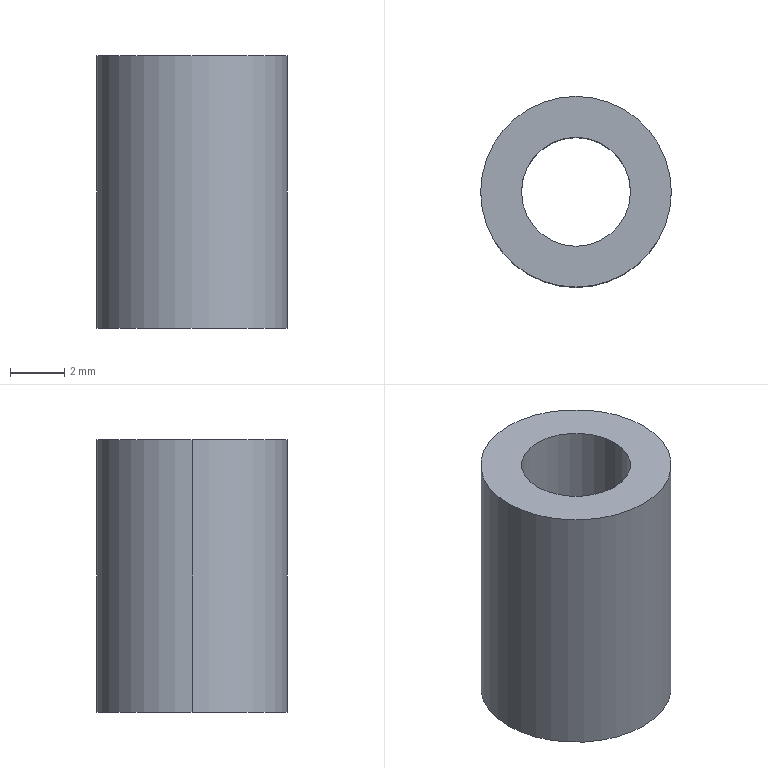Part | STEP file | MANIFOLD_SOLID_BREP_312481-2 | 1 solid | 6 faces | box 7 x 7 x 10 mm | volume 259.181 mm3 | cylinder 4 | plane 2 | commonest cylinder face diameters 4 x2 7 x2
STEP:
#1=CARTESIAN_POINT('',(-23.5,58.,-348.));
#2=VERTEX_POINT('',#1);
#3=CARTESIAN_POINT('',(-16.5,58.,-348.));
#4=VERTEX_POINT('',#3);
#5=CARTESIAN_POINT('',(-20.,58.,-348.));
#6=DIRECTION('',(0.,0.,-1.));
#7=DIRECTION('',(-1.,0.,0.));
#8=AXIS2_PLACEMENT_3D('',#5,#6,#7);
#9=CIRCLE('',#8,3.5);
#10=EDGE_CURVE('',#2,#4,#9,.T.);
#11=ORIENTED_EDGE('',*,*,#10,.T.);
#12=CARTESIAN_POINT('',(-16.5,58.,-358.));
#13=VERTEX_POINT('',#12);
#14=CARTESIAN_POINT('',(-16.5,58.,-348.));
#15=DIRECTION('',(0.,0.,-1.));
#16=VECTOR('',#15,1000.);
#17=LINE('',#14,#16);
#18=EDGE_CURVE('',#4,#13,#17,.T.);
#19=ORIENTED_EDGE('',*,*,#18,.T.);
#20=CARTESIAN_POINT('',(-23.5,58.,-358.));
#21=VERTEX_POINT('',#20);
#22=CARTESIAN_POINT('',(-20.,58.,-358.));
#23=DIRECTION('',(0.,0.,1.));
#24=DIRECTION('',(-1.,0.,0.));
#25=AXIS2_PLACEMENT_3D('',#22,#23,#24);
#26=CIRCLE('',#25,3.5);
#27=EDGE_CURVE('',#13,#21,#26,.T.);
#28=ORIENTED_EDGE('',*,*,#27,.T.);
#29=CARTESIAN_POINT('',(-23.5,58.,-348.));
#30=DIRECTION('',(0.,0.,-1.));
#31=VECTOR('',#30,1000.);
#32=LINE('',#29,#31);
#33=EDGE_CURVE('',#2,#21,#32,.T.);
#34=ORIENTED_EDGE('',*,*,#33,.F.);
#35=EDGE_LOOP('',(#11,#19,#28,#34));
#36=FACE_OUTER_BOUND('',#35,.T.);
#37=CARTESIAN_POINT('',(-20.,58.,-348.));
#38=DIRECTION('',(0.,0.,-1.));
#39=DIRECTION('',(-1.,0.,0.));
#40=AXIS2_PLACEMENT_3D('',#37,#38,#39);
#41=CYLINDRICAL_SURFACE('',#40,3.5);
#42=ADVANCED_FACE('',(#36),#41,.T.);
#43=CARTESIAN_POINT('',(-18.,58.,-348.));
#44=VERTEX_POINT('',#43);
#45=CARTESIAN_POINT('',(-22.,58.,-348.));
#46=VERTEX_POINT('',#45);
#47=CARTESIAN_POINT('',(-20.,58.,-348.));
#48=DIRECTION('',(0.,0.,-1.));
#49=DIRECTION('',(-1.,0.,0.));
#50=AXIS2_PLACEMENT_3D('',#47,#48,#49);
#51=CIRCLE('',#50,2.);
#52=EDGE_CURVE('',#44,#46,#51,.T.);
#53=ORIENTED_EDGE('',*,*,#52,.F.);
#54=CARTESIAN_POINT('',(-18.,58.,-358.));
#55=VERTEX_POINT('',#54);
#56=CARTESIAN_POINT('',(-18.,58.,-348.));
#57=DIRECTION('',(0.,0.,-1.));
#58=VECTOR('',#57,1000.);
#59=LINE('',#56,#58);
#60=EDGE_CURVE('',#44,#55,#59,.T.);
#61=ORIENTED_EDGE('',*,*,#60,.T.);
#62=CARTESIAN_POINT('',(-22.,58.,-358.));
#63=VERTEX_POINT('',#62);
#64=CARTESIAN_POINT('',(-20.,58.,-358.));
#65=DIRECTION('',(0.,0.,-1.));
#66=DIRECTION('',(-1.,0.,0.));
#67=AXIS2_PLACEMENT_3D('',#64,#65,#66);
#68=CIRCLE('',#67,2.);
#69=EDGE_CURVE('',#55,#63,#68,.T.);
#70=ORIENTED_EDGE('',*,*,#69,.T.);
#71=CARTESIAN_POINT('',(-22.,58.,-348.));
#72=DIRECTION('',(0.,0.,-1.));
#73=VECTOR('',#72,1000.);
#74=LINE('',#71,#73);
#75=EDGE_CURVE('',#46,#63,#74,.T.);
#76=ORIENTED_EDGE('',*,*,#75,.F.);
#77=EDGE_LOOP('',(#53,#61,#70,#76));
#78=FACE_OUTER_BOUND('',#77,.T.);
#79=CARTESIAN_POINT('',(-20.,58.,-348.));
#80=DIRECTION('',(0.,0.,-1.));
#81=DIRECTION('',(-1.,0.,0.));
#82=AXIS2_PLACEMENT_3D('',#79,#80,#81);
#83=CYLINDRICAL_SURFACE('',#82,2.);
#84=ADVANCED_FACE('',(#78),#83,.F.);
#85=ORIENTED_EDGE('',*,*,#18,.F.);
#86=CARTESIAN_POINT('',(-20.,58.,-348.));
#87=DIRECTION('',(0.,0.,-1.));
#88=DIRECTION('',(-1.,0.,0.));
#89=AXIS2_PLACEMENT_3D('',#86,#87,#88);
#90=CIRCLE('',#89,3.5);
#91=EDGE_CURVE('',#4,#2,#90,.T.);
#92=ORIENTED_EDGE('',*,*,#91,.T.);
#93=ORIENTED_EDGE('',*,*,#33,.T.);
#94=CARTESIAN_POINT('',(-20.,58.,-358.));
#95=DIRECTION('',(0.,0.,1.));
#96=DIRECTION('',(-1.,0.,0.));
#97=AXIS2_PLACEMENT_3D('',#94,#95,#96);
#98=CIRCLE('',#97,3.5);
#99=EDGE_CURVE('',#21,#13,#98,.T.);
#100=ORIENTED_EDGE('',*,*,#99,.T.);
#101=EDGE_LOOP('',(#85,#92,#93,#100));
#102=FACE_OUTER_BOUND('',#101,.T.);
#103=CARTESIAN_POINT('',(-20.,58.,-348.));
#104=DIRECTION('',(0.,0.,-1.));
#105=DIRECTION('',(-1.,0.,0.));
#106=AXIS2_PLACEMENT_3D('',#103,#104,#105);
#107=CYLINDRICAL_SURFACE('',#106,3.5);
#108=ADVANCED_FACE('',(#102),#107,.T.);
#109=CARTESIAN_POINT('',(-20.,58.,-348.));
#110=DIRECTION('',(0.,0.,-1.));
#111=DIRECTION('',(-1.,0.,0.));
#112=AXIS2_PLACEMENT_3D('',#109,#110,#111);
#113=CIRCLE('',#112,2.);
#114=EDGE_CURVE('',#46,#44,#113,.T.);
#115=ORIENTED_EDGE('',*,*,#114,.T.);
#116=ORIENTED_EDGE('',*,*,#52,.T.);
#117=EDGE_LOOP('',(#115,#116));
#118=FACE_BOUND('',#117,.T.);
#119=ORIENTED_EDGE('',*,*,#10,.F.);
#120=ORIENTED_EDGE('',*,*,#91,.F.);
#121=EDGE_LOOP('',(#119,#120));
#122=FACE_OUTER_BOUND('',#121,.T.);
#123=CARTESIAN_POINT('',(-20.,60.75,-348.));
#124=DIRECTION('',(0.,0.,1.));
#125=DIRECTION('',(1.,0.,0.));
#126=AXIS2_PLACEMENT_3D('',#123,#124,#125);
#127=PLANE('',#126);
#128=ADVANCED_FACE('',(#118,#122),#127,.T.);
#129=CARTESIAN_POINT('',(-20.,58.,-358.));
#130=DIRECTION('',(0.,0.,-1.));
#131=DIRECTION('',(-1.,0.,0.));
#132=AXIS2_PLACEMENT_3D('',#129,#130,#131);
#133=CIRCLE('',#132,2.);
#134=EDGE_CURVE('',#63,#55,#133,.T.);
#135=ORIENTED_EDGE('',*,*,#134,.F.);
#136=ORIENTED_EDGE('',*,*,#69,.F.);
#137=EDGE_LOOP('',(#135,#136));
#138=FACE_BOUND('',#137,.T.);
#139=ORIENTED_EDGE('',*,*,#99,.F.);
#140=ORIENTED_EDGE('',*,*,#27,.F.);
#141=EDGE_LOOP('',(#139,#140));
#142=FACE_OUTER_BOUND('',#141,.T.);
#143=CARTESIAN_POINT('',(-20.,60.75,-358.));
#144=DIRECTION('',(0.,0.,1.));
#145=DIRECTION('',(1.,0.,0.));
#146=AXIS2_PLACEMENT_3D('',#143,#144,#145);
#147=PLANE('',#146);
#148=ADVANCED_FACE('',(#138,#142),#147,.F.);
#149=ORIENTED_EDGE('',*,*,#60,.F.);
#150=ORIENTED_EDGE('',*,*,#114,.F.);
#151=ORIENTED_EDGE('',*,*,#75,.T.);
#152=ORIENTED_EDGE('',*,*,#134,.T.);
#153=EDGE_LOOP('',(#149,#150,#151,#152));
#154=FACE_OUTER_BOUND('',#153,.T.);
#155=CARTESIAN_POINT('',(-20.,58.,-348.));
#156=DIRECTION('',(0.,0.,-1.));
#157=DIRECTION('',(-1.,0.,0.));
#158=AXIS2_PLACEMENT_3D('',#155,#156,#157);
#159=CYLINDRICAL_SURFACE('',#158,2.);
#160=ADVANCED_FACE('',(#154),#159,.F.);
#161=CLOSED_SHELL('',(#42,#84,#108,#128,#148,#160));
#162=MANIFOLD_SOLID_BREP('',#161);
#163=CARTESIAN_POINT('',(0.,0.,0.));
#164=DIRECTION('',(0.,0.,1.));
#165=DIRECTION('',(1.,0.,0.));
#166=AXIS2_PLACEMENT_3D('',#163,#164,#165);
#167=(LENGTH_UNIT()NAMED_UNIT(*)SI_UNIT(.MILLI.,.METRE.));
#168=UNCERTAINTY_MEASURE_WITH_UNIT(LENGTH_MEASURE(0.00001),#167,'','');
#169=(NAMED_UNIT(*)PLANE_ANGLE_UNIT()SI_UNIT($,.RADIAN.));
#170=(NAMED_UNIT(*)SI_UNIT($,.STERADIAN.)SOLID_ANGLE_UNIT());
#171=(GEOMETRIC_REPRESENTATION_CONTEXT(3)GLOBAL_UNCERTAINTY_ASSIGNED_CONTEXT((#168))GLOBAL_UNIT_ASSIGNED_CONTEXT((#167,#169,#170))REPRESENTATION_CONTEXT('',''));
#172=ADVANCED_BREP_SHAPE_REPRESENTATION('',(#162,#166),#171);